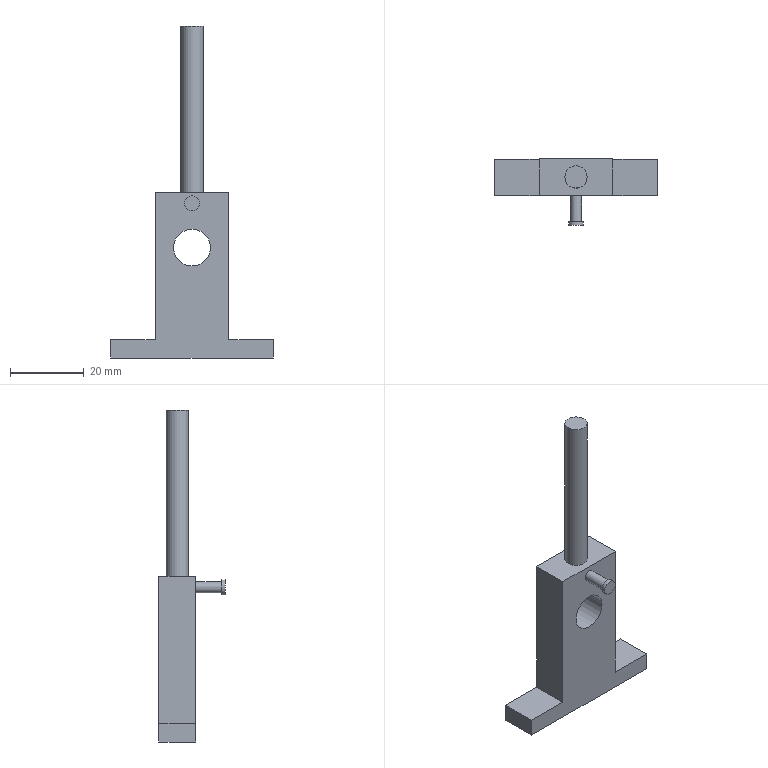Part | NX | features DATUM_CSYS 5, EXTRUDE 4, SKETCH 4 | 1 solid | 17 faces | box 44 x 18 x 89.9 mm | volume 10705 mm3 | plane 13 | cylinder 4 | commonest cylinder face diameters 3 x1 4 x1 6 x1 10 x1
STEP:
#1=CARTESIAN_POINT('',(-22.,5.,4.9));
#2=VERTEX_POINT('',#1);
#3=CARTESIAN_POINT('',(-22.,5.,0.));
#4=VERTEX_POINT('',#3);
#5=CARTESIAN_POINT('',(-22.,5.,4.9));
#6=DIRECTION('',(0.,0.,-1.));
#7=VECTOR('',#6,1000.);
#8=LINE('',#5,#7);
#9=EDGE_CURVE('',#2,#4,#8,.T.);
#10=ORIENTED_EDGE('',*,*,#9,.T.);
#11=CARTESIAN_POINT('',(-22.,-5.,0.));
#12=VERTEX_POINT('',#11);
#13=CARTESIAN_POINT('',(-22.,-5.,0.));
#14=DIRECTION('',(0.,1.,0.));
#15=VECTOR('',#14,1000.);
#16=LINE('',#13,#15);
#17=EDGE_CURVE('',#12,#4,#16,.T.);
#18=ORIENTED_EDGE('',*,*,#17,.F.);
#19=CARTESIAN_POINT('',(-22.,-5.,4.9));
#20=VERTEX_POINT('',#19);
#21=CARTESIAN_POINT('',(-22.,-5.,4.9));
#22=DIRECTION('',(0.,0.,-1.));
#23=VECTOR('',#22,1000.);
#24=LINE('',#21,#23);
#25=EDGE_CURVE('',#20,#12,#24,.T.);
#26=ORIENTED_EDGE('',*,*,#25,.F.);
#27=CARTESIAN_POINT('',(-22.,-5.,4.9));
#28=DIRECTION('',(0.,1.,0.));
#29=VECTOR('',#28,1000.);
#30=LINE('',#27,#29);
#31=EDGE_CURVE('',#20,#2,#30,.T.);
#32=ORIENTED_EDGE('',*,*,#31,.T.);
#33=EDGE_LOOP('',(#10,#18,#26,#32));
#34=FACE_BOUND('',#33,.T.);
#35=CARTESIAN_POINT('',(-22.,-5.,4.9));
#36=DIRECTION('',(1.,0.,0.));
#37=DIRECTION('',(0.,0.,-1.));
#38=AXIS2_PLACEMENT_3D('',#35,#36,#37);
#39=PLANE('',#38);
#40=ADVANCED_FACE('',(#34),#39,.F.);
#41=CARTESIAN_POINT('',(22.,5.,0.));
#42=VERTEX_POINT('',#41);
#43=CARTESIAN_POINT('',(0.,5.,0.));
#44=DIRECTION('',(1.,0.,0.));
#45=VECTOR('',#44,1000.);
#46=LINE('',#43,#45);
#47=EDGE_CURVE('',#4,#42,#46,.T.);
#48=ORIENTED_EDGE('',*,*,#47,.T.);
#49=CARTESIAN_POINT('',(22.,-5.,0.));
#50=VERTEX_POINT('',#49);
#51=CARTESIAN_POINT('',(22.,-5.,0.));
#52=DIRECTION('',(0.,1.,0.));
#53=VECTOR('',#52,1000.);
#54=LINE('',#51,#53);
#55=EDGE_CURVE('',#50,#42,#54,.T.);
#56=ORIENTED_EDGE('',*,*,#55,.F.);
#57=CARTESIAN_POINT('',(-22.,-5.,0.));
#58=DIRECTION('',(1.,0.,0.));
#59=VECTOR('',#58,1000.);
#60=LINE('',#57,#59);
#61=EDGE_CURVE('',#12,#50,#60,.T.);
#62=ORIENTED_EDGE('',*,*,#61,.F.);
#63=ORIENTED_EDGE('',*,*,#17,.T.);
#64=EDGE_LOOP('',(#48,#56,#62,#63));
#65=FACE_BOUND('',#64,.T.);
#66=CARTESIAN_POINT('',(0.,-5.,0.));
#67=DIRECTION('',(0.,0.,1.));
#68=DIRECTION('',(1.,0.,0.));
#69=AXIS2_PLACEMENT_3D('',#66,#67,#68);
#70=PLANE('',#69);
#71=ADVANCED_FACE('',(#65),#70,.F.);
#72=CARTESIAN_POINT('',(22.,5.,4.9));
#73=VERTEX_POINT('',#72);
#74=CARTESIAN_POINT('',(22.,5.,0.));
#75=DIRECTION('',(0.,0.,1.));
#76=VECTOR('',#75,1000.);
#77=LINE('',#74,#76);
#78=EDGE_CURVE('',#42,#73,#77,.T.);
#79=ORIENTED_EDGE('',*,*,#78,.T.);
#80=CARTESIAN_POINT('',(22.,-5.,4.9));
#81=VERTEX_POINT('',#80);
#82=CARTESIAN_POINT('',(22.,-5.,4.9));
#83=DIRECTION('',(0.,1.,0.));
#84=VECTOR('',#83,1000.);
#85=LINE('',#82,#84);
#86=EDGE_CURVE('',#81,#73,#85,.T.);
#87=ORIENTED_EDGE('',*,*,#86,.F.);
#88=CARTESIAN_POINT('',(22.,-5.,0.));
#89=DIRECTION('',(0.,0.,1.));
#90=VECTOR('',#89,1000.);
#91=LINE('',#88,#90);
#92=EDGE_CURVE('',#50,#81,#91,.T.);
#93=ORIENTED_EDGE('',*,*,#92,.F.);
#94=ORIENTED_EDGE('',*,*,#55,.T.);
#95=EDGE_LOOP('',(#79,#87,#93,#94));
#96=FACE_BOUND('',#95,.T.);
#97=CARTESIAN_POINT('',(22.,-5.,0.));
#98=DIRECTION('',(-1.,0.,0.));
#99=DIRECTION('',(0.,0.,1.));
#100=AXIS2_PLACEMENT_3D('',#97,#98,#99);
#101=PLANE('',#100);
#102=ADVANCED_FACE('',(#96),#101,.F.);
#103=CARTESIAN_POINT('',(10.,5.,4.9));
#104=VERTEX_POINT('',#103);
#105=CARTESIAN_POINT('',(22.,5.,4.9));
#106=DIRECTION('',(-1.,0.,0.));
#107=VECTOR('',#106,1000.);
#108=LINE('',#105,#107);
#109=EDGE_CURVE('',#73,#104,#108,.T.);
#110=ORIENTED_EDGE('',*,*,#109,.T.);
#111=CARTESIAN_POINT('',(10.,-5.,4.9));
#112=VERTEX_POINT('',#111);
#113=CARTESIAN_POINT('',(10.,-5.,4.9));
#114=DIRECTION('',(0.,1.,0.));
#115=VECTOR('',#114,1000.);
#116=LINE('',#113,#115);
#117=EDGE_CURVE('',#112,#104,#116,.T.);
#118=ORIENTED_EDGE('',*,*,#117,.F.);
#119=CARTESIAN_POINT('',(22.,-5.,4.9));
#120=DIRECTION('',(-1.,0.,0.));
#121=VECTOR('',#120,1000.);
#122=LINE('',#119,#121);
#123=EDGE_CURVE('',#81,#112,#122,.T.);
#124=ORIENTED_EDGE('',*,*,#123,.F.);
#125=ORIENTED_EDGE('',*,*,#86,.T.);
#126=EDGE_LOOP('',(#110,#118,#124,#125));
#127=FACE_BOUND('',#126,.T.);
#128=CARTESIAN_POINT('',(22.,-5.,4.9));
#129=DIRECTION('',(0.,0.,-1.));
#130=DIRECTION('',(-1.,0.,0.));
#131=AXIS2_PLACEMENT_3D('',#128,#129,#130);
#132=PLANE('',#131);
#133=ADVANCED_FACE('',(#127),#132,.F.);
#134=CARTESIAN_POINT('',(10.,5.,44.9));
#135=VERTEX_POINT('',#134);
#136=CARTESIAN_POINT('',(10.,5.,4.9));
#137=DIRECTION('',(0.,0.,1.));
#138=VECTOR('',#137,1000.);
#139=LINE('',#136,#138);
#140=EDGE_CURVE('',#104,#135,#139,.T.);
#141=ORIENTED_EDGE('',*,*,#140,.T.);
#142=CARTESIAN_POINT('',(10.,-5.,44.9));
#143=VERTEX_POINT('',#142);
#144=CARTESIAN_POINT('',(10.,-5.,44.9));
#145=DIRECTION('',(0.,1.,0.));
#146=VECTOR('',#145,1000.);
#147=LINE('',#144,#146);
#148=EDGE_CURVE('',#143,#135,#147,.T.);
#149=ORIENTED_EDGE('',*,*,#148,.F.);
#150=CARTESIAN_POINT('',(10.,-5.,4.9));
#151=DIRECTION('',(0.,0.,1.));
#152=VECTOR('',#151,1000.);
#153=LINE('',#150,#152);
#154=EDGE_CURVE('',#112,#143,#153,.T.);
#155=ORIENTED_EDGE('',*,*,#154,.F.);
#156=ORIENTED_EDGE('',*,*,#117,.T.);
#157=EDGE_LOOP('',(#141,#149,#155,#156));
#158=FACE_BOUND('',#157,.T.);
#159=CARTESIAN_POINT('',(10.,-5.,4.9));
#160=DIRECTION('',(-1.,0.,0.));
#161=DIRECTION('',(0.,0.,1.));
#162=AXIS2_PLACEMENT_3D('',#159,#160,#161);
#163=PLANE('',#162);
#164=ADVANCED_FACE('',(#158),#163,.F.);
#165=CARTESIAN_POINT('',(-3.,0.,44.9));
#166=VERTEX_POINT('',#165);
#167=CARTESIAN_POINT('',(0.,0.,44.9));
#168=DIRECTION('',(0.,0.,-1.));
#169=DIRECTION('',(-1.,0.,0.));
#170=AXIS2_PLACEMENT_3D('',#167,#168,#169);
#171=CIRCLE('',#170,3.);
#172=EDGE_CURVE('',#166,#166,#171,.T.);
#173=ORIENTED_EDGE('',*,*,#172,.T.);
#174=EDGE_LOOP('',(#173));
#175=FACE_BOUND('',#174,.T.);
#176=CARTESIAN_POINT('',(-10.,5.,44.9));
#177=VERTEX_POINT('',#176);
#178=CARTESIAN_POINT('',(0.,5.,44.9));
#179=DIRECTION('',(-1.,0.,0.));
#180=VECTOR('',#179,1000.);
#181=LINE('',#178,#180);
#182=EDGE_CURVE('',#135,#177,#181,.T.);
#183=ORIENTED_EDGE('',*,*,#182,.T.);
#184=CARTESIAN_POINT('',(-10.,-5.,44.9));
#185=VERTEX_POINT('',#184);
#186=CARTESIAN_POINT('',(-10.,-5.,44.9));
#187=DIRECTION('',(0.,1.,0.));
#188=VECTOR('',#187,1000.);
#189=LINE('',#186,#188);
#190=EDGE_CURVE('',#185,#177,#189,.T.);
#191=ORIENTED_EDGE('',*,*,#190,.F.);
#192=CARTESIAN_POINT('',(10.,-5.,44.9));
#193=DIRECTION('',(-1.,0.,0.));
#194=VECTOR('',#193,1000.);
#195=LINE('',#192,#194);
#196=EDGE_CURVE('',#143,#185,#195,.T.);
#197=ORIENTED_EDGE('',*,*,#196,.F.);
#198=ORIENTED_EDGE('',*,*,#148,.T.);
#199=EDGE_LOOP('',(#183,#191,#197,#198));
#200=FACE_BOUND('',#199,.T.);
#201=CARTESIAN_POINT('',(0.,-5.,44.9));
#202=DIRECTION('',(0.,0.,-1.));
#203=DIRECTION('',(-1.,0.,0.));
#204=AXIS2_PLACEMENT_3D('',#201,#202,#203);
#205=PLANE('',#204);
#206=ADVANCED_FACE('',(#175,#200),#205,.F.);
#207=CARTESIAN_POINT('',(-10.,5.,4.9));
#208=VERTEX_POINT('',#207);
#209=CARTESIAN_POINT('',(-10.,5.,44.9));
#210=DIRECTION('',(0.,0.,-1.));
#211=VECTOR('',#210,1000.);
#212=LINE('',#209,#211);
#213=EDGE_CURVE('',#177,#208,#212,.T.);
#214=ORIENTED_EDGE('',*,*,#213,.T.);
#215=CARTESIAN_POINT('',(-10.,-5.,4.9));
#216=VERTEX_POINT('',#215);
#217=CARTESIAN_POINT('',(-10.,-5.,4.9));
#218=DIRECTION('',(0.,1.,0.));
#219=VECTOR('',#218,1000.);
#220=LINE('',#217,#219);
#221=EDGE_CURVE('',#216,#208,#220,.T.);
#222=ORIENTED_EDGE('',*,*,#221,.F.);
#223=CARTESIAN_POINT('',(-10.,-5.,44.9));
#224=DIRECTION('',(0.,0.,-1.));
#225=VECTOR('',#224,1000.);
#226=LINE('',#223,#225);
#227=EDGE_CURVE('',#185,#216,#226,.T.);
#228=ORIENTED_EDGE('',*,*,#227,.F.);
#229=ORIENTED_EDGE('',*,*,#190,.T.);
#230=EDGE_LOOP('',(#214,#222,#228,#229));
#231=FACE_BOUND('',#230,.T.);
#232=CARTESIAN_POINT('',(-10.,-5.,44.9));
#233=DIRECTION('',(1.,0.,0.));
#234=DIRECTION('',(0.,0.,-1.));
#235=AXIS2_PLACEMENT_3D('',#232,#233,#234);
#236=PLANE('',#235);
#237=ADVANCED_FACE('',(#231),#236,.F.);
#238=CARTESIAN_POINT('',(-10.,5.,4.9));
#239=DIRECTION('',(-1.,0.,0.));
#240=VECTOR('',#239,1000.);
#241=LINE('',#238,#240);
#242=EDGE_CURVE('',#208,#2,#241,.T.);
#243=ORIENTED_EDGE('',*,*,#242,.T.);
#244=ORIENTED_EDGE('',*,*,#31,.F.);
#245=CARTESIAN_POINT('',(-10.,-5.,4.9));
#246=DIRECTION('',(-1.,0.,0.));
#247=VECTOR('',#246,1000.);
#248=LINE('',#245,#247);
#249=EDGE_CURVE('',#216,#20,#248,.T.);
#250=ORIENTED_EDGE('',*,*,#249,.F.);
#251=ORIENTED_EDGE('',*,*,#221,.T.);
#252=EDGE_LOOP('',(#243,#244,#250,#251));
#253=FACE_BOUND('',#252,.T.);
#254=CARTESIAN_POINT('',(-10.,-5.,4.9));
#255=DIRECTION('',(0.,0.,-1.));
#256=DIRECTION('',(-1.,0.,0.));
#257=AXIS2_PLACEMENT_3D('',#254,#255,#256);
#258=PLANE('',#257);
#259=ADVANCED_FACE('',(#253),#258,.F.);
#260=CARTESIAN_POINT('',(5.,-5.,29.9));
#261=VERTEX_POINT('',#260);
#262=CARTESIAN_POINT('',(0.,-5.,29.9));
#263=DIRECTION('',(0.,1.,0.));
#264=DIRECTION('',(1.,0.,0.));
#265=AXIS2_PLACEMENT_3D('',#262,#263,#264);
#266=CIRCLE('',#265,5.);
#267=EDGE_CURVE('',#261,#261,#266,.T.);
#268=ORIENTED_EDGE('',*,*,#267,.F.);
#269=EDGE_LOOP('',(#268));
#270=FACE_BOUND('',#269,.T.);
#271=CARTESIAN_POINT('',(5.,5.,29.9));
#272=VERTEX_POINT('',#271);
#273=CARTESIAN_POINT('',(0.,5.,29.9));
#274=DIRECTION('',(0.,1.,0.));
#275=DIRECTION('',(1.,0.,0.));
#276=AXIS2_PLACEMENT_3D('',#273,#274,#275);
#277=CIRCLE('',#276,5.);
#278=EDGE_CURVE('',#272,#272,#277,.T.);
#279=ORIENTED_EDGE('',*,*,#278,.T.);
#280=EDGE_LOOP('',(#279));
#281=FACE_BOUND('',#280,.T.);
#282=CARTESIAN_POINT('',(0.,-5.,29.9));
#283=DIRECTION('',(0.,1.,0.));
#284=DIRECTION('',(0.,0.,1.));
#285=AXIS2_PLACEMENT_3D('',#282,#283,#284);
#286=CYLINDRICAL_SURFACE('',#285,5.);
#287=ADVANCED_FACE('',(#270,#281),#286,.F.);
#288=CARTESIAN_POINT('',(1.5,-5.,41.9));
#289=VERTEX_POINT('',#288);
#290=CARTESIAN_POINT('',(0.,-5.,41.9));
#291=DIRECTION('',(0.,1.,0.));
#292=DIRECTION('',(1.,0.,0.));
#293=AXIS2_PLACEMENT_3D('',#290,#291,#292);
#294=CIRCLE('',#293,1.5);
#295=EDGE_CURVE('',#289,#289,#294,.T.);
#296=ORIENTED_EDGE('',*,*,#295,.T.);
#297=EDGE_LOOP('',(#296));
#298=FACE_BOUND('',#297,.T.);
#299=ORIENTED_EDGE('',*,*,#25,.T.);
#300=ORIENTED_EDGE('',*,*,#61,.T.);
#301=ORIENTED_EDGE('',*,*,#92,.T.);
#302=ORIENTED_EDGE('',*,*,#123,.T.);
#303=ORIENTED_EDGE('',*,*,#154,.T.);
#304=ORIENTED_EDGE('',*,*,#196,.T.);
#305=ORIENTED_EDGE('',*,*,#227,.T.);
#306=ORIENTED_EDGE('',*,*,#249,.T.);
#307=EDGE_LOOP('',(#299,#300,#301,#302,#303,#304,#305,#306));
#308=FACE_BOUND('',#307,.T.);
#309=ORIENTED_EDGE('',*,*,#267,.T.);
#310=EDGE_LOOP('',(#309));
#311=FACE_BOUND('',#310,.T.);
#312=CARTESIAN_POINT('',(0.,-5.,29.9));
#313=DIRECTION('',(0.,1.,0.));
#314=DIRECTION('',(0.,0.,1.));
#315=AXIS2_PLACEMENT_3D('',#312,#313,#314);
#316=PLANE('',#315);
#317=ADVANCED_FACE('',(#298,#308,#311),#316,.F.);
#318=ORIENTED_EDGE('',*,*,#9,.F.);
#319=ORIENTED_EDGE('',*,*,#242,.F.);
#320=ORIENTED_EDGE('',*,*,#213,.F.);
#321=ORIENTED_EDGE('',*,*,#182,.F.);
#322=ORIENTED_EDGE('',*,*,#140,.F.);
#323=ORIENTED_EDGE('',*,*,#109,.F.);
#324=ORIENTED_EDGE('',*,*,#78,.F.);
#325=ORIENTED_EDGE('',*,*,#47,.F.);
#326=EDGE_LOOP('',(#318,#319,#320,#321,#322,#323,#324,#325));
#327=FACE_BOUND('',#326,.T.);
#328=ORIENTED_EDGE('',*,*,#278,.F.);
#329=EDGE_LOOP('',(#328));
#330=FACE_BOUND('',#329,.T.);
#331=CARTESIAN_POINT('',(0.,5.,29.9));
#332=DIRECTION('',(0.,1.,0.));
#333=DIRECTION('',(0.,0.,1.));
#334=AXIS2_PLACEMENT_3D('',#331,#332,#333);
#335=PLANE('',#334);
#336=ADVANCED_FACE('',(#327,#330),#335,.T.);
#337=CARTESIAN_POINT('',(3.,0.,89.9));
#338=VERTEX_POINT('',#337);
#339=CARTESIAN_POINT('',(0.,0.,89.9));
#340=DIRECTION('',(0.,0.,1.));
#341=DIRECTION('',(1.,0.,0.));
#342=AXIS2_PLACEMENT_3D('',#339,#340,#341);
#343=CIRCLE('',#342,3.);
#344=EDGE_CURVE('',#338,#338,#343,.T.);
#345=ORIENTED_EDGE('',*,*,#344,.F.);
#346=EDGE_LOOP('',(#345));
#347=FACE_BOUND('',#346,.T.);
#348=ORIENTED_EDGE('',*,*,#172,.F.);
#349=EDGE_LOOP('',(#348));
#350=FACE_BOUND('',#349,.T.);
#351=CARTESIAN_POINT('',(0.,0.,89.9));
#352=DIRECTION('',(0.,0.,-1.));
#353=DIRECTION('',(-1.,0.,0.));
#354=AXIS2_PLACEMENT_3D('',#351,#352,#353);
#355=CYLINDRICAL_SURFACE('',#354,3.);
#356=ADVANCED_FACE('',(#347,#350),#355,.T.);
#357=ORIENTED_EDGE('',*,*,#344,.T.);
#358=EDGE_LOOP('',(#357));
#359=FACE_BOUND('',#358,.T.);
#360=CARTESIAN_POINT('',(0.,0.,89.9));
#361=DIRECTION('',(0.,0.,1.));
#362=DIRECTION('',(1.,0.,0.));
#363=AXIS2_PLACEMENT_3D('',#360,#361,#362);
#364=PLANE('',#363);
#365=ADVANCED_FACE('',(#359),#364,.T.);
#366=CARTESIAN_POINT('',(1.5,-12.,41.9));
#367=VERTEX_POINT('',#366);
#368=CARTESIAN_POINT('',(0.,-12.,41.9));
#369=DIRECTION('',(0.,1.,0.));
#370=DIRECTION('',(1.,0.,0.));
#371=AXIS2_PLACEMENT_3D('',#368,#369,#370);
#372=CIRCLE('',#371,1.5);
#373=EDGE_CURVE('',#367,#367,#372,.T.);
#374=ORIENTED_EDGE('',*,*,#373,.T.);
#375=EDGE_LOOP('',(#374));
#376=FACE_BOUND('',#375,.T.);
#377=ORIENTED_EDGE('',*,*,#295,.F.);
#378=EDGE_LOOP('',(#377));
#379=FACE_BOUND('',#378,.T.);
#380=CARTESIAN_POINT('',(0.,-12.,41.9));
#381=DIRECTION('',(0.,1.,0.));
#382=DIRECTION('',(0.,0.,1.));
#383=AXIS2_PLACEMENT_3D('',#380,#381,#382);
#384=CYLINDRICAL_SURFACE('',#383,1.5);
#385=ADVANCED_FACE('',(#376,#379),#384,.T.);
#386=CARTESIAN_POINT('',(-2.,-13.,41.9));
#387=VERTEX_POINT('',#386);
#388=CARTESIAN_POINT('',(0.,-13.,41.9));
#389=DIRECTION('',(0.,1.,0.));
#390=DIRECTION('',(-1.,0.,0.));
#391=AXIS2_PLACEMENT_3D('',#388,#389,#390);
#392=CIRCLE('',#391,2.);
#393=EDGE_CURVE('',#387,#387,#392,.T.);
#394=ORIENTED_EDGE('',*,*,#393,.T.);
#395=EDGE_LOOP('',(#394));
#396=FACE_BOUND('',#395,.T.);
#397=CARTESIAN_POINT('',(-2.,-12.,41.9));
#398=VERTEX_POINT('',#397);
#399=CARTESIAN_POINT('',(0.,-12.,41.9));
#400=DIRECTION('',(0.,1.,0.));
#401=DIRECTION('',(-1.,0.,0.));
#402=AXIS2_PLACEMENT_3D('',#399,#400,#401);
#403=CIRCLE('',#402,2.);
#404=EDGE_CURVE('',#398,#398,#403,.T.);
#405=ORIENTED_EDGE('',*,*,#404,.F.);
#406=EDGE_LOOP('',(#405));
#407=FACE_BOUND('',#406,.T.);
#408=CARTESIAN_POINT('',(0.,-13.,41.9));
#409=DIRECTION('',(0.,1.,0.));
#410=DIRECTION('',(0.,0.,1.));
#411=AXIS2_PLACEMENT_3D('',#408,#409,#410);
#412=CYLINDRICAL_SURFACE('',#411,2.);
#413=ADVANCED_FACE('',(#396,#407),#412,.T.);
#414=ORIENTED_EDGE('',*,*,#393,.F.);
#415=EDGE_LOOP('',(#414));
#416=FACE_BOUND('',#415,.T.);
#417=CARTESIAN_POINT('',(0.,-13.,41.9));
#418=DIRECTION('',(0.,1.,0.));
#419=DIRECTION('',(0.,0.,1.));
#420=AXIS2_PLACEMENT_3D('',#417,#418,#419);
#421=PLANE('',#420);
#422=ADVANCED_FACE('',(#416),#421,.F.);
#423=ORIENTED_EDGE('',*,*,#373,.F.);
#424=EDGE_LOOP('',(#423));
#425=FACE_BOUND('',#424,.T.);
#426=ORIENTED_EDGE('',*,*,#404,.T.);
#427=EDGE_LOOP('',(#426));
#428=FACE_BOUND('',#427,.T.);
#429=CARTESIAN_POINT('',(0.,-12.,41.9));
#430=DIRECTION('',(0.,1.,0.));
#431=DIRECTION('',(0.,0.,1.));
#432=AXIS2_PLACEMENT_3D('',#429,#430,#431);
#433=PLANE('',#432);
#434=ADVANCED_FACE('',(#425,#428),#433,.T.);
#435=CLOSED_SHELL('',(#40,#71,#102,#133,#164,#206,#237,#259,#287,#317,#336,#356,#365,#385,#413,#422,#434));
#436=MANIFOLD_SOLID_BREP('',#435);
#437=(LENGTH_UNIT()NAMED_UNIT(*)SI_UNIT(.MILLI.,.METRE.));
#438=UNCERTAINTY_MEASURE_WITH_UNIT(LENGTH_MEASURE(0.00001),#437,'','');
#439=(NAMED_UNIT(*)PLANE_ANGLE_UNIT()SI_UNIT($,.RADIAN.));
#440=(NAMED_UNIT(*)SI_UNIT($,.STERADIAN.)SOLID_ANGLE_UNIT());
#441=(GEOMETRIC_REPRESENTATION_CONTEXT(3)GLOBAL_UNCERTAINTY_ASSIGNED_CONTEXT((#438))GLOBAL_UNIT_ASSIGNED_CONTEXT((#437,#439,#440))REPRESENTATION_CONTEXT('',''));
#442=ADVANCED_BREP_SHAPE_REPRESENTATION('',(#436),#441);